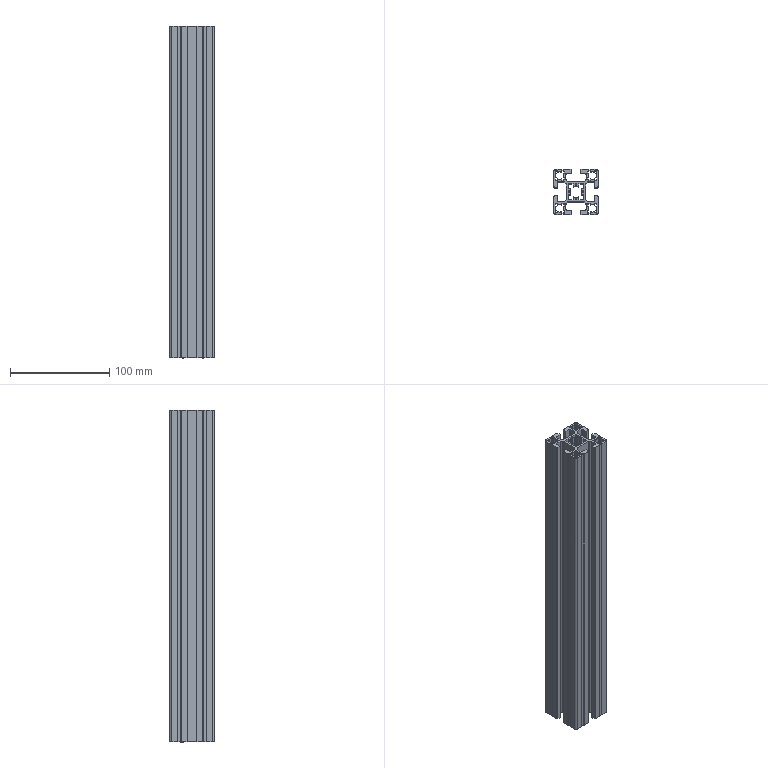Part | STEP file | 4545-390 Al (side support) | 1 solid | 262 faces | box 45 x 45 x 335 mm | volume 232439 mm3 | plane 186 | cylinder 76 | commonest cylinder face diameters 2 x44 8 x20 12 x8 4 x4